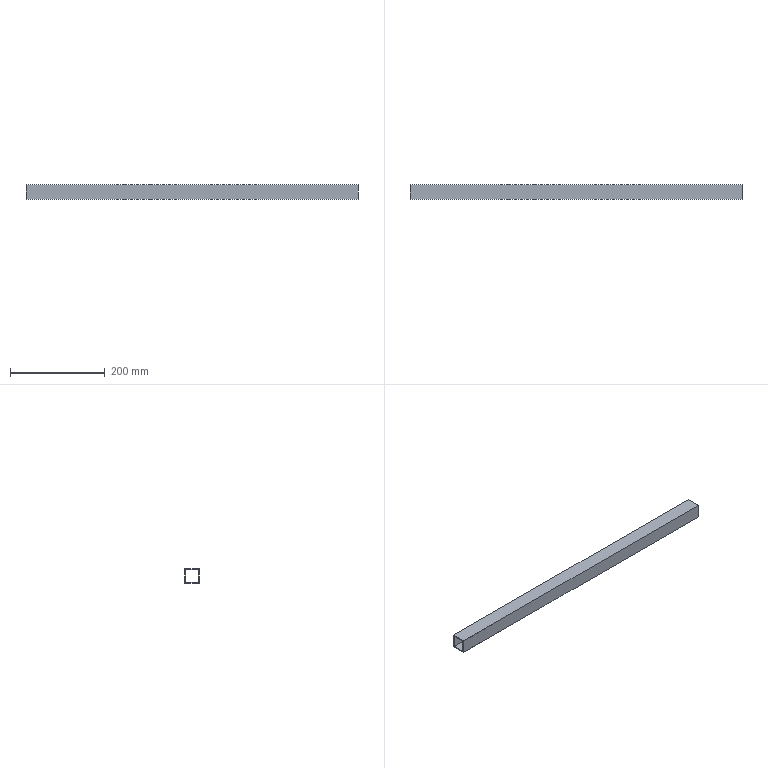Part | NX | features solid 2 | 1 solid | 10 faces | box 700 x 30 x 30 mm | volume 156800 mm3 | plane 10
STEP:
#1=CARTESIAN_POINT('',(350.,-330.,-60.));
#2=VERTEX_POINT('',#1);
#3=CARTESIAN_POINT('',(350.,-300.,-60.));
#4=VERTEX_POINT('',#3);
#5=CARTESIAN_POINT('',(350.,-387.5,-60.));
#6=DIRECTION('',(0.,1.,0.));
#7=VECTOR('',#6,1000.);
#8=LINE('',#5,#7);
#9=EDGE_CURVE('',#2,#4,#8,.T.);
#10=ORIENTED_EDGE('',*,*,#9,.T.);
#11=CARTESIAN_POINT('',(350.,-300.,-30.));
#12=VERTEX_POINT('',#11);
#13=CARTESIAN_POINT('',(350.,-300.,-30.));
#14=DIRECTION('',(0.,0.,-1.));
#15=VECTOR('',#14,1000.);
#16=LINE('',#13,#15);
#17=EDGE_CURVE('',#12,#4,#16,.T.);
#18=ORIENTED_EDGE('',*,*,#17,.F.);
#19=CARTESIAN_POINT('',(350.,-330.,-30.));
#20=VERTEX_POINT('',#19);
#21=CARTESIAN_POINT('',(350.,-387.5,-30.));
#22=DIRECTION('',(0.,1.,0.));
#23=VECTOR('',#22,1000.);
#24=LINE('',#21,#23);
#25=EDGE_CURVE('',#20,#12,#24,.T.);
#26=ORIENTED_EDGE('',*,*,#25,.F.);
#27=CARTESIAN_POINT('',(350.,-330.,-30.));
#28=DIRECTION('',(0.,0.,-1.));
#29=VECTOR('',#28,1000.);
#30=LINE('',#27,#29);
#31=EDGE_CURVE('',#20,#2,#30,.T.);
#32=ORIENTED_EDGE('',*,*,#31,.T.);
#33=EDGE_LOOP('',(#10,#18,#26,#32));
#34=FACE_BOUND('',#33,.T.);
#35=CARTESIAN_POINT('',(350.,-328.,-32.));
#36=VERTEX_POINT('',#35);
#37=CARTESIAN_POINT('',(350.,-328.,-58.));
#38=VERTEX_POINT('',#37);
#39=CARTESIAN_POINT('',(350.,-328.,-30.));
#40=DIRECTION('',(0.,0.,-1.));
#41=VECTOR('',#40,1000.);
#42=LINE('',#39,#41);
#43=EDGE_CURVE('',#36,#38,#42,.T.);
#44=ORIENTED_EDGE('',*,*,#43,.F.);
#45=CARTESIAN_POINT('',(350.,-302.,-32.));
#46=VERTEX_POINT('',#45);
#47=CARTESIAN_POINT('',(350.,-387.5,-32.));
#48=DIRECTION('',(0.,1.,0.));
#49=VECTOR('',#48,1000.);
#50=LINE('',#47,#49);
#51=EDGE_CURVE('',#36,#46,#50,.T.);
#52=ORIENTED_EDGE('',*,*,#51,.T.);
#53=CARTESIAN_POINT('',(350.,-302.,-58.));
#54=VERTEX_POINT('',#53);
#55=CARTESIAN_POINT('',(350.,-302.,-30.));
#56=DIRECTION('',(0.,0.,-1.));
#57=VECTOR('',#56,1000.);
#58=LINE('',#55,#57);
#59=EDGE_CURVE('',#46,#54,#58,.T.);
#60=ORIENTED_EDGE('',*,*,#59,.T.);
#61=CARTESIAN_POINT('',(350.,-387.5,-58.));
#62=DIRECTION('',(0.,1.,0.));
#63=VECTOR('',#62,1000.);
#64=LINE('',#61,#63);
#65=EDGE_CURVE('',#38,#54,#64,.T.);
#66=ORIENTED_EDGE('',*,*,#65,.F.);
#67=EDGE_LOOP('',(#44,#52,#60,#66));
#68=FACE_BOUND('',#67,.T.);
#69=CARTESIAN_POINT('',(350.,-620.,-30.));
#70=DIRECTION('',(1.,0.,0.));
#71=DIRECTION('',(0.,0.,1.));
#72=AXIS2_PLACEMENT_3D('',#69,#70,#71);
#73=PLANE('',#72);
#74=ADVANCED_FACE('',(#34,#68),#73,.T.);
#75=CARTESIAN_POINT('',(-350.,-330.,-60.));
#76=VERTEX_POINT('',#75);
#77=CARTESIAN_POINT('',(320.,-330.,-60.));
#78=DIRECTION('',(-1.,0.,0.));
#79=VECTOR('',#78,1000.);
#80=LINE('',#77,#79);
#81=EDGE_CURVE('',#2,#76,#80,.T.);
#82=ORIENTED_EDGE('',*,*,#81,.F.);
#83=ORIENTED_EDGE('',*,*,#31,.F.);
#84=CARTESIAN_POINT('',(-350.,-330.,-30.));
#85=VERTEX_POINT('',#84);
#86=CARTESIAN_POINT('',(320.,-330.,-30.));
#87=DIRECTION('',(-1.,0.,0.));
#88=VECTOR('',#87,1000.);
#89=LINE('',#86,#88);
#90=EDGE_CURVE('',#20,#85,#89,.T.);
#91=ORIENTED_EDGE('',*,*,#90,.T.);
#92=CARTESIAN_POINT('',(-350.,-330.,-30.));
#93=DIRECTION('',(0.,0.,-1.));
#94=VECTOR('',#93,1000.);
#95=LINE('',#92,#94);
#96=EDGE_CURVE('',#85,#76,#95,.T.);
#97=ORIENTED_EDGE('',*,*,#96,.T.);
#98=EDGE_LOOP('',(#82,#83,#91,#97));
#99=FACE_BOUND('',#98,.T.);
#100=CARTESIAN_POINT('',(320.,-330.,-30.));
#101=DIRECTION('',(0.,1.,0.));
#102=DIRECTION('',(0.,0.,1.));
#103=AXIS2_PLACEMENT_3D('',#100,#101,#102);
#104=PLANE('',#103);
#105=ADVANCED_FACE('',(#99),#104,.F.);
#106=CARTESIAN_POINT('',(-350.,-300.,-60.));
#107=VERTEX_POINT('',#106);
#108=CARTESIAN_POINT('',(350.,-300.,-60.));
#109=DIRECTION('',(-1.,0.,0.));
#110=VECTOR('',#109,1000.);
#111=LINE('',#108,#110);
#112=EDGE_CURVE('',#4,#107,#111,.T.);
#113=ORIENTED_EDGE('',*,*,#112,.T.);
#114=CARTESIAN_POINT('',(-350.,-300.,-30.));
#115=VERTEX_POINT('',#114);
#116=CARTESIAN_POINT('',(-350.,-300.,-30.));
#117=DIRECTION('',(0.,0.,-1.));
#118=VECTOR('',#117,1000.);
#119=LINE('',#116,#118);
#120=EDGE_CURVE('',#115,#107,#119,.T.);
#121=ORIENTED_EDGE('',*,*,#120,.F.);
#122=CARTESIAN_POINT('',(350.,-300.,-30.));
#123=DIRECTION('',(-1.,0.,0.));
#124=VECTOR('',#123,1000.);
#125=LINE('',#122,#124);
#126=EDGE_CURVE('',#12,#115,#125,.T.);
#127=ORIENTED_EDGE('',*,*,#126,.F.);
#128=ORIENTED_EDGE('',*,*,#17,.T.);
#129=EDGE_LOOP('',(#113,#121,#127,#128));
#130=FACE_BOUND('',#129,.T.);
#131=CARTESIAN_POINT('',(350.,-300.,-30.));
#132=DIRECTION('',(0.,1.,0.));
#133=DIRECTION('',(0.,0.,1.));
#134=AXIS2_PLACEMENT_3D('',#131,#132,#133);
#135=PLANE('',#134);
#136=ADVANCED_FACE('',(#130),#135,.T.);
#137=ORIENTED_EDGE('',*,*,#25,.T.);
#138=ORIENTED_EDGE('',*,*,#126,.T.);
#139=CARTESIAN_POINT('',(-350.,-620.,-30.));
#140=DIRECTION('',(0.,1.,0.));
#141=VECTOR('',#140,1000.);
#142=LINE('',#139,#141);
#143=EDGE_CURVE('',#85,#115,#142,.T.);
#144=ORIENTED_EDGE('',*,*,#143,.F.);
#145=ORIENTED_EDGE('',*,*,#90,.F.);
#146=EDGE_LOOP('',(#137,#138,#144,#145));
#147=FACE_BOUND('',#146,.T.);
#148=CARTESIAN_POINT('',(247.5,-387.5,-30.));
#149=DIRECTION('',(0.,0.,1.));
#150=DIRECTION('',(-1.,0.,0.));
#151=AXIS2_PLACEMENT_3D('',#148,#149,#150);
#152=PLANE('',#151);
#153=ADVANCED_FACE('',(#147),#152,.T.);
#154=ORIENTED_EDGE('',*,*,#9,.F.);
#155=ORIENTED_EDGE('',*,*,#81,.T.);
#156=CARTESIAN_POINT('',(-350.,-620.,-60.));
#157=DIRECTION('',(0.,1.,0.));
#158=VECTOR('',#157,1000.);
#159=LINE('',#156,#158);
#160=EDGE_CURVE('',#76,#107,#159,.T.);
#161=ORIENTED_EDGE('',*,*,#160,.T.);
#162=ORIENTED_EDGE('',*,*,#112,.F.);
#163=EDGE_LOOP('',(#154,#155,#161,#162));
#164=FACE_BOUND('',#163,.T.);
#165=CARTESIAN_POINT('',(247.5,-387.5,-60.));
#166=DIRECTION('',(0.,0.,1.));
#167=DIRECTION('',(-1.,0.,0.));
#168=AXIS2_PLACEMENT_3D('',#165,#166,#167);
#169=PLANE('',#168);
#170=ADVANCED_FACE('',(#164),#169,.F.);
#171=CARTESIAN_POINT('',(-350.,-328.,-58.));
#172=VERTEX_POINT('',#171);
#173=CARTESIAN_POINT('',(320.,-328.,-58.));
#174=DIRECTION('',(-1.,0.,0.));
#175=VECTOR('',#174,1000.);
#176=LINE('',#173,#175);
#177=EDGE_CURVE('',#38,#172,#176,.T.);
#178=ORIENTED_EDGE('',*,*,#177,.T.);
#179=CARTESIAN_POINT('',(-350.,-328.,-32.));
#180=VERTEX_POINT('',#179);
#181=CARTESIAN_POINT('',(-350.,-328.,-30.));
#182=DIRECTION('',(0.,0.,-1.));
#183=VECTOR('',#182,1000.);
#184=LINE('',#181,#183);
#185=EDGE_CURVE('',#180,#172,#184,.T.);
#186=ORIENTED_EDGE('',*,*,#185,.F.);
#187=CARTESIAN_POINT('',(320.,-328.,-32.));
#188=DIRECTION('',(-1.,0.,0.));
#189=VECTOR('',#188,1000.);
#190=LINE('',#187,#189);
#191=EDGE_CURVE('',#36,#180,#190,.T.);
#192=ORIENTED_EDGE('',*,*,#191,.F.);
#193=ORIENTED_EDGE('',*,*,#43,.T.);
#194=EDGE_LOOP('',(#178,#186,#192,#193));
#195=FACE_BOUND('',#194,.T.);
#196=CARTESIAN_POINT('',(320.,-328.,-30.));
#197=DIRECTION('',(0.,1.,0.));
#198=DIRECTION('',(0.,0.,1.));
#199=AXIS2_PLACEMENT_3D('',#196,#197,#198);
#200=PLANE('',#199);
#201=ADVANCED_FACE('',(#195),#200,.T.);
#202=CARTESIAN_POINT('',(-350.,-302.,-58.));
#203=VERTEX_POINT('',#202);
#204=CARTESIAN_POINT('',(350.,-302.,-58.));
#205=DIRECTION('',(-1.,0.,0.));
#206=VECTOR('',#205,1000.);
#207=LINE('',#204,#206);
#208=EDGE_CURVE('',#54,#203,#207,.T.);
#209=ORIENTED_EDGE('',*,*,#208,.F.);
#210=ORIENTED_EDGE('',*,*,#59,.F.);
#211=CARTESIAN_POINT('',(-350.,-302.,-32.));
#212=VERTEX_POINT('',#211);
#213=CARTESIAN_POINT('',(350.,-302.,-32.));
#214=DIRECTION('',(-1.,0.,0.));
#215=VECTOR('',#214,1000.);
#216=LINE('',#213,#215);
#217=EDGE_CURVE('',#46,#212,#216,.T.);
#218=ORIENTED_EDGE('',*,*,#217,.T.);
#219=CARTESIAN_POINT('',(-350.,-302.,-30.));
#220=DIRECTION('',(0.,0.,-1.));
#221=VECTOR('',#220,1000.);
#222=LINE('',#219,#221);
#223=EDGE_CURVE('',#212,#203,#222,.T.);
#224=ORIENTED_EDGE('',*,*,#223,.T.);
#225=EDGE_LOOP('',(#209,#210,#218,#224));
#226=FACE_BOUND('',#225,.T.);
#227=CARTESIAN_POINT('',(350.,-302.,-30.));
#228=DIRECTION('',(0.,1.,0.));
#229=DIRECTION('',(0.,0.,1.));
#230=AXIS2_PLACEMENT_3D('',#227,#228,#229);
#231=PLANE('',#230);
#232=ADVANCED_FACE('',(#226),#231,.F.);
#233=ORIENTED_EDGE('',*,*,#51,.F.);
#234=ORIENTED_EDGE('',*,*,#191,.T.);
#235=CARTESIAN_POINT('',(-350.,-620.,-32.));
#236=DIRECTION('',(0.,1.,0.));
#237=VECTOR('',#236,1000.);
#238=LINE('',#235,#237);
#239=EDGE_CURVE('',#180,#212,#238,.T.);
#240=ORIENTED_EDGE('',*,*,#239,.T.);
#241=ORIENTED_EDGE('',*,*,#217,.F.);
#242=EDGE_LOOP('',(#233,#234,#240,#241));
#243=FACE_BOUND('',#242,.T.);
#244=CARTESIAN_POINT('',(247.5,-387.5,-32.));
#245=DIRECTION('',(0.,0.,1.));
#246=DIRECTION('',(-1.,0.,0.));
#247=AXIS2_PLACEMENT_3D('',#244,#245,#246);
#248=PLANE('',#247);
#249=ADVANCED_FACE('',(#243),#248,.F.);
#250=ORIENTED_EDGE('',*,*,#65,.T.);
#251=ORIENTED_EDGE('',*,*,#208,.T.);
#252=CARTESIAN_POINT('',(-350.,-620.,-58.));
#253=DIRECTION('',(0.,1.,0.));
#254=VECTOR('',#253,1000.);
#255=LINE('',#252,#254);
#256=EDGE_CURVE('',#172,#203,#255,.T.);
#257=ORIENTED_EDGE('',*,*,#256,.F.);
#258=ORIENTED_EDGE('',*,*,#177,.F.);
#259=EDGE_LOOP('',(#250,#251,#257,#258));
#260=FACE_BOUND('',#259,.T.);
#261=CARTESIAN_POINT('',(247.5,-387.5,-58.));
#262=DIRECTION('',(0.,0.,1.));
#263=DIRECTION('',(-1.,0.,0.));
#264=AXIS2_PLACEMENT_3D('',#261,#262,#263);
#265=PLANE('',#264);
#266=ADVANCED_FACE('',(#260),#265,.T.);
#267=ORIENTED_EDGE('',*,*,#160,.F.);
#268=ORIENTED_EDGE('',*,*,#96,.F.);
#269=ORIENTED_EDGE('',*,*,#143,.T.);
#270=ORIENTED_EDGE('',*,*,#120,.T.);
#271=EDGE_LOOP('',(#267,#268,#269,#270));
#272=FACE_BOUND('',#271,.T.);
#273=ORIENTED_EDGE('',*,*,#185,.T.);
#274=ORIENTED_EDGE('',*,*,#256,.T.);
#275=ORIENTED_EDGE('',*,*,#223,.F.);
#276=ORIENTED_EDGE('',*,*,#239,.F.);
#277=EDGE_LOOP('',(#273,#274,#275,#276));
#278=FACE_BOUND('',#277,.T.);
#279=CARTESIAN_POINT('',(-350.,-620.,-30.));
#280=DIRECTION('',(-1.,0.,0.));
#281=DIRECTION('',(0.,0.,1.));
#282=AXIS2_PLACEMENT_3D('',#279,#280,#281);
#283=PLANE('',#282);
#284=ADVANCED_FACE('',(#272,#278),#283,.T.);
#285=CLOSED_SHELL('',(#74,#105,#136,#153,#170,#201,#232,#249,#266,#284));
#286=MANIFOLD_SOLID_BREP('',#285);
#287=(LENGTH_UNIT()NAMED_UNIT(*)SI_UNIT(.MILLI.,.METRE.));
#288=UNCERTAINTY_MEASURE_WITH_UNIT(LENGTH_MEASURE(0.00001),#287,'','');
#289=(NAMED_UNIT(*)PLANE_ANGLE_UNIT()SI_UNIT($,.RADIAN.));
#290=(NAMED_UNIT(*)SI_UNIT($,.STERADIAN.)SOLID_ANGLE_UNIT());
#291=(GEOMETRIC_REPRESENTATION_CONTEXT(3)GLOBAL_UNCERTAINTY_ASSIGNED_CONTEXT((#288))GLOBAL_UNIT_ASSIGNED_CONTEXT((#287,#289,#290))REPRESENTATION_CONTEXT('',''));
#292=ADVANCED_BREP_SHAPE_REPRESENTATION('',(#286),#291);